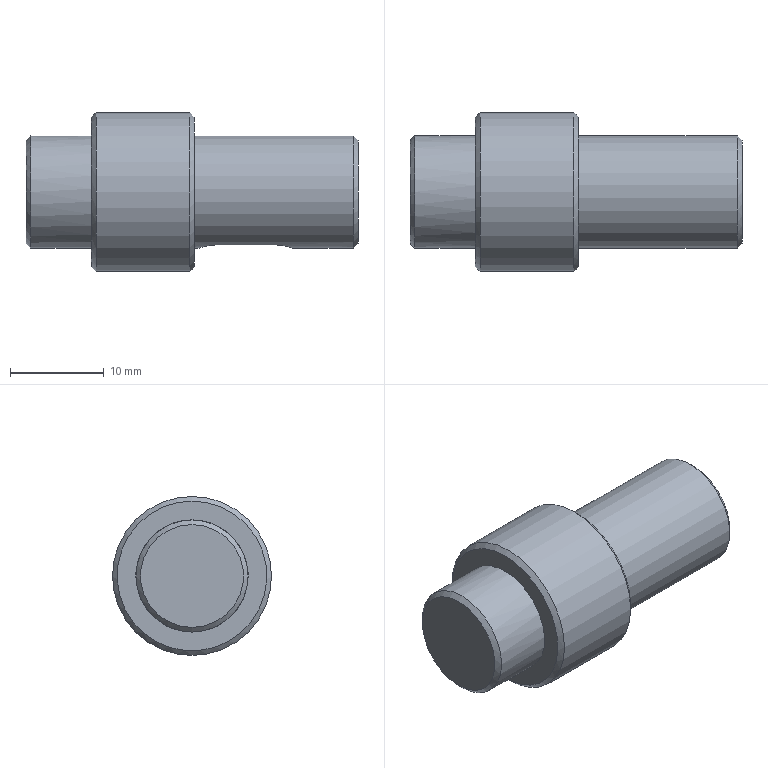Part | NX | features BREP 1 | 1 solid | 16 faces | box 35.5 x 17 x 17 mm | volume 5158 mm3 | plane 7 | cylinder 5 | cone 4 | commonest cylinder face diameters 4 x2 12 x2 17 x1
STEP:
#1=CARTESIAN_POINT('',(35.,0.,-6.));
#2=VERTEX_POINT('',#1);
#3=CARTESIAN_POINT('',(35.,0.,0.));
#4=DIRECTION('',(-1.,0.,0.));
#5=DIRECTION('',(0.,0.,-1.));
#6=AXIS2_PLACEMENT_3D('',#3,#4,#5);
#7=CIRCLE('',#6,6.);
#8=EDGE_CURVE('',#2,#2,#7,.T.);
#9=ORIENTED_EDGE('',*,*,#8,.F.);
#10=EDGE_LOOP('',(#9));
#11=FACE_BOUND('',#10,.T.);
#12=CARTESIAN_POINT('',(35.5,0.,-5.5));
#13=VERTEX_POINT('',#12);
#14=CARTESIAN_POINT('',(35.5,0.,0.));
#15=DIRECTION('',(1.,0.,0.));
#16=DIRECTION('',(0.,0.,-1.));
#17=AXIS2_PLACEMENT_3D('',#14,#15,#16);
#18=CIRCLE('',#17,5.5);
#19=EDGE_CURVE('',#13,#13,#18,.T.);
#20=ORIENTED_EDGE('',*,*,#19,.F.);
#21=EDGE_LOOP('',(#20));
#22=FACE_BOUND('',#21,.T.);
#23=CARTESIAN_POINT('',(35.5,0.,0.));
#24=DIRECTION('',(-1.,0.,0.));
#25=DIRECTION('',(0.,0.,1.));
#26=AXIS2_PLACEMENT_3D('',#23,#24,#25);
#27=CONICAL_SURFACE('',#26,5.5,0.7854);
#28=ADVANCED_FACE('',(#11,#22),#27,.T.);
#29=CARTESIAN_POINT('',(17.5,0.,-8.5));
#30=VERTEX_POINT('',#29);
#31=CARTESIAN_POINT('',(17.5,0.,0.));
#32=DIRECTION('',(-1.,0.,0.));
#33=DIRECTION('',(0.,0.,-1.));
#34=AXIS2_PLACEMENT_3D('',#31,#32,#33);
#35=CIRCLE('',#34,8.5);
#36=EDGE_CURVE('',#30,#30,#35,.T.);
#37=ORIENTED_EDGE('',*,*,#36,.F.);
#38=EDGE_LOOP('',(#37));
#39=FACE_BOUND('',#38,.T.);
#40=CARTESIAN_POINT('',(18.,0.,-8.));
#41=VERTEX_POINT('',#40);
#42=CARTESIAN_POINT('',(18.,0.,0.));
#43=DIRECTION('',(1.,0.,0.));
#44=DIRECTION('',(0.,0.,-1.));
#45=AXIS2_PLACEMENT_3D('',#42,#43,#44);
#46=CIRCLE('',#45,8.);
#47=EDGE_CURVE('',#41,#41,#46,.T.);
#48=ORIENTED_EDGE('',*,*,#47,.F.);
#49=EDGE_LOOP('',(#48));
#50=FACE_BOUND('',#49,.T.);
#51=CARTESIAN_POINT('',(18.,0.,0.));
#52=DIRECTION('',(-1.,0.,0.));
#53=DIRECTION('',(0.,0.,1.));
#54=AXIS2_PLACEMENT_3D('',#51,#52,#53);
#55=CONICAL_SURFACE('',#54,8.,0.7854);
#56=ADVANCED_FACE('',(#39,#50),#55,.T.);
#57=CARTESIAN_POINT('',(7.5,0.,8.5));
#58=VERTEX_POINT('',#57);
#59=CARTESIAN_POINT('',(7.5,0.,0.));
#60=DIRECTION('',(1.,0.,0.));
#61=DIRECTION('',(0.,0.,1.));
#62=AXIS2_PLACEMENT_3D('',#59,#60,#61);
#63=CIRCLE('',#62,8.5);
#64=EDGE_CURVE('',#58,#58,#63,.T.);
#65=ORIENTED_EDGE('',*,*,#64,.F.);
#66=EDGE_LOOP('',(#65));
#67=FACE_BOUND('',#66,.T.);
#68=CARTESIAN_POINT('',(7.,0.,8.));
#69=VERTEX_POINT('',#68);
#70=CARTESIAN_POINT('',(7.,0.,0.));
#71=DIRECTION('',(-1.,0.,0.));
#72=DIRECTION('',(0.,0.,1.));
#73=AXIS2_PLACEMENT_3D('',#70,#71,#72);
#74=CIRCLE('',#73,8.);
#75=EDGE_CURVE('',#69,#69,#74,.T.);
#76=ORIENTED_EDGE('',*,*,#75,.F.);
#77=EDGE_LOOP('',(#76));
#78=FACE_BOUND('',#77,.T.);
#79=CARTESIAN_POINT('',(7.5,0.,0.));
#80=DIRECTION('',(1.,0.,0.));
#81=DIRECTION('',(0.,0.,-1.));
#82=AXIS2_PLACEMENT_3D('',#79,#80,#81);
#83=CONICAL_SURFACE('',#82,8.5,0.7854);
#84=ADVANCED_FACE('',(#67,#78),#83,.T.);
#85=CARTESIAN_POINT('',(0.5,0.,6.));
#86=VERTEX_POINT('',#85);
#87=CARTESIAN_POINT('',(0.5,0.,0.));
#88=DIRECTION('',(1.,0.,0.));
#89=DIRECTION('',(0.,0.,1.));
#90=AXIS2_PLACEMENT_3D('',#87,#88,#89);
#91=CIRCLE('',#90,6.);
#92=EDGE_CURVE('',#86,#86,#91,.T.);
#93=ORIENTED_EDGE('',*,*,#92,.F.);
#94=EDGE_LOOP('',(#93));
#95=FACE_BOUND('',#94,.T.);
#96=CARTESIAN_POINT('',(0.,0.,5.5));
#97=VERTEX_POINT('',#96);
#98=CARTESIAN_POINT('',(0.,0.,0.));
#99=DIRECTION('',(-1.,0.,0.));
#100=DIRECTION('',(0.,0.,1.));
#101=AXIS2_PLACEMENT_3D('',#98,#99,#100);
#102=CIRCLE('',#101,5.5);
#103=EDGE_CURVE('',#97,#97,#102,.T.);
#104=ORIENTED_EDGE('',*,*,#103,.F.);
#105=EDGE_LOOP('',(#104));
#106=FACE_BOUND('',#105,.T.);
#107=CARTESIAN_POINT('',(0.5,0.,0.));
#108=DIRECTION('',(1.,0.,0.));
#109=DIRECTION('',(0.,0.,-1.));
#110=AXIS2_PLACEMENT_3D('',#107,#108,#109);
#111=CONICAL_SURFACE('',#110,6.,0.7854);
#112=ADVANCED_FACE('',(#95,#106),#111,.T.);
#113=CARTESIAN_POINT('',(20.5,-2.,-3.5));
#114=VERTEX_POINT('',#113);
#115=CARTESIAN_POINT('',(20.5,2.,-3.5));
#116=VERTEX_POINT('',#115);
#117=CARTESIAN_POINT('',(20.5,0.,-3.5));
#118=DIRECTION('',(0.,0.,-1.));
#119=DIRECTION('',(1.,0.,0.));
#120=AXIS2_PLACEMENT_3D('',#117,#118,#119);
#121=CIRCLE('',#120,2.);
#122=EDGE_CURVE('',#114,#116,#121,.T.);
#123=ORIENTED_EDGE('',*,*,#122,.F.);
#124=CARTESIAN_POINT('',(20.5,-2.,-5.657));
#125=VERTEX_POINT('',#124);
#126=CARTESIAN_POINT('',(20.5,-2.,-3.5));
#127=DIRECTION('',(0.,0.,-1.));
#128=VECTOR('',#127,1000.);
#129=LINE('',#126,#128);
#130=EDGE_CURVE('',#114,#125,#129,.T.);
#131=ORIENTED_EDGE('',*,*,#130,.T.);
#132=CARTESIAN_POINT('',(20.5,2.,-5.657));
#133=VERTEX_POINT('',#132);
#134=CARTESIAN_POINT('',(20.5,-2.,-5.657));
#135=CARTESIAN_POINT('',(19.967,-2.,-5.657));
#136=CARTESIAN_POINT('',(18.938,-1.567,-5.833));
#137=CARTESIAN_POINT('',(18.281,-0.003461,-6.083));
#138=CARTESIAN_POINT('',(18.937,1.568,-5.834));
#139=CARTESIAN_POINT('',(19.967,2.,-5.657));
#140=CARTESIAN_POINT('',(20.5,2.,-5.657));
#141=B_SPLINE_CURVE_WITH_KNOTS('',3,(#134,#135,#136,#137,#138,#139,#140),.UNSPECIFIED.,.F.,.F.,(4,1,1,1,4),(0.,0.001574,0.003148,0.004722,0.006296),.UNSPECIFIED.);
#142=EDGE_CURVE('',#125,#133,#141,.T.);
#143=ORIENTED_EDGE('',*,*,#142,.T.);
#144=CARTESIAN_POINT('',(20.5,2.,-3.5));
#145=DIRECTION('',(0.,0.,-1.));
#146=VECTOR('',#145,1000.);
#147=LINE('',#144,#146);
#148=EDGE_CURVE('',#116,#133,#147,.T.);
#149=ORIENTED_EDGE('',*,*,#148,.F.);
#150=EDGE_LOOP('',(#123,#131,#143,#149));
#151=FACE_BOUND('',#150,.T.);
#152=CARTESIAN_POINT('',(20.5,0.,-3.5));
#153=DIRECTION('',(0.,0.,-1.));
#154=DIRECTION('',(-1.,0.,0.));
#155=AXIS2_PLACEMENT_3D('',#152,#153,#154);
#156=CYLINDRICAL_SURFACE('',#155,2.);
#157=ADVANCED_FACE('',(#151),#156,.F.);
#158=ORIENTED_EDGE('',*,*,#8,.T.);
#159=EDGE_LOOP('',(#158));
#160=FACE_BOUND('',#159,.T.);
#161=ORIENTED_EDGE('',*,*,#142,.F.);
#162=CARTESIAN_POINT('',(26.5,-2.,-5.657));
#163=VERTEX_POINT('',#162);
#164=CARTESIAN_POINT('',(35.5,-2.,-5.657));
#165=DIRECTION('',(-1.,0.,0.));
#166=VECTOR('',#165,1000.);
#167=LINE('',#164,#166);
#168=EDGE_CURVE('',#163,#125,#167,.T.);
#169=ORIENTED_EDGE('',*,*,#168,.F.);
#170=CARTESIAN_POINT('',(26.5,2.,-5.657));
#171=VERTEX_POINT('',#170);
#172=CARTESIAN_POINT('',(26.5,2.,-5.657));
#173=CARTESIAN_POINT('',(27.033,2.,-5.657));
#174=CARTESIAN_POINT('',(28.062,1.567,-5.833));
#175=CARTESIAN_POINT('',(28.719,0.003461,-6.083));
#176=CARTESIAN_POINT('',(28.063,-1.568,-5.834));
#177=CARTESIAN_POINT('',(27.033,-2.,-5.657));
#178=CARTESIAN_POINT('',(26.5,-2.,-5.657));
#179=B_SPLINE_CURVE_WITH_KNOTS('',3,(#172,#173,#174,#175,#176,#177,#178),.UNSPECIFIED.,.F.,.F.,(4,1,1,1,4),(0.,0.001574,0.003148,0.004722,0.006296),.UNSPECIFIED.);
#180=EDGE_CURVE('',#171,#163,#179,.T.);
#181=ORIENTED_EDGE('',*,*,#180,.F.);
#182=CARTESIAN_POINT('',(35.5,2.,-5.657));
#183=DIRECTION('',(1.,0.,0.));
#184=VECTOR('',#183,1000.);
#185=LINE('',#182,#184);
#186=EDGE_CURVE('',#133,#171,#185,.T.);
#187=ORIENTED_EDGE('',*,*,#186,.F.);
#188=EDGE_LOOP('',(#161,#169,#181,#187));
#189=FACE_BOUND('',#188,.T.);
#190=CARTESIAN_POINT('',(18.,0.,-6.));
#191=VERTEX_POINT('',#190);
#192=CARTESIAN_POINT('',(18.,0.,0.));
#193=DIRECTION('',(1.,0.,0.));
#194=DIRECTION('',(0.,0.,-1.));
#195=AXIS2_PLACEMENT_3D('',#192,#193,#194);
#196=CIRCLE('',#195,6.);
#197=EDGE_CURVE('',#191,#191,#196,.T.);
#198=ORIENTED_EDGE('',*,*,#197,.T.);
#199=EDGE_LOOP('',(#198));
#200=FACE_BOUND('',#199,.T.);
#201=CARTESIAN_POINT('',(35.5,0.,0.));
#202=DIRECTION('',(1.,0.,0.));
#203=DIRECTION('',(0.,0.,-1.));
#204=AXIS2_PLACEMENT_3D('',#201,#202,#203);
#205=CYLINDRICAL_SURFACE('',#204,6.);
#206=ADVANCED_FACE('',(#160,#189,#200),#205,.T.);
#207=ORIENTED_EDGE('',*,*,#36,.T.);
#208=EDGE_LOOP('',(#207));
#209=FACE_BOUND('',#208,.T.);
#210=ORIENTED_EDGE('',*,*,#64,.T.);
#211=EDGE_LOOP('',(#210));
#212=FACE_BOUND('',#211,.T.);
#213=CARTESIAN_POINT('',(35.5,0.,0.));
#214=DIRECTION('',(1.,0.,0.));
#215=DIRECTION('',(0.,0.,-1.));
#216=AXIS2_PLACEMENT_3D('',#213,#214,#215);
#217=CYLINDRICAL_SURFACE('',#216,8.5);
#218=ADVANCED_FACE('',(#209,#212),#217,.T.);
#219=CARTESIAN_POINT('',(7.,0.,-6.));
#220=VERTEX_POINT('',#219);
#221=CARTESIAN_POINT('',(7.,0.,0.));
#222=DIRECTION('',(1.,0.,0.));
#223=DIRECTION('',(0.,0.,-1.));
#224=AXIS2_PLACEMENT_3D('',#221,#222,#223);
#225=CIRCLE('',#224,6.);
#226=EDGE_CURVE('',#220,#220,#225,.T.);
#227=ORIENTED_EDGE('',*,*,#226,.F.);
#228=EDGE_LOOP('',(#227));
#229=FACE_BOUND('',#228,.T.);
#230=ORIENTED_EDGE('',*,*,#92,.T.);
#231=EDGE_LOOP('',(#230));
#232=FACE_BOUND('',#231,.T.);
#233=CARTESIAN_POINT('',(35.5,0.,0.));
#234=DIRECTION('',(1.,0.,0.));
#235=DIRECTION('',(0.,0.,-1.));
#236=AXIS2_PLACEMENT_3D('',#233,#234,#235);
#237=CYLINDRICAL_SURFACE('',#236,6.);
#238=ADVANCED_FACE('',(#229,#232),#237,.T.);
#239=ORIENTED_EDGE('',*,*,#103,.T.);
#240=EDGE_LOOP('',(#239));
#241=FACE_BOUND('',#240,.T.);
#242=CARTESIAN_POINT('',(0.,0.,0.));
#243=DIRECTION('',(-1.,0.,0.));
#244=DIRECTION('',(0.,0.,1.));
#245=AXIS2_PLACEMENT_3D('',#242,#243,#244);
#246=PLANE('',#245);
#247=ADVANCED_FACE('',(#241),#246,.T.);
#248=ORIENTED_EDGE('',*,*,#75,.T.);
#249=EDGE_LOOP('',(#248));
#250=FACE_BOUND('',#249,.T.);
#251=ORIENTED_EDGE('',*,*,#226,.T.);
#252=EDGE_LOOP('',(#251));
#253=FACE_BOUND('',#252,.T.);
#254=CARTESIAN_POINT('',(7.,6.,0.));
#255=DIRECTION('',(-1.,0.,0.));
#256=DIRECTION('',(0.,0.,1.));
#257=AXIS2_PLACEMENT_3D('',#254,#255,#256);
#258=PLANE('',#257);
#259=ADVANCED_FACE('',(#250,#253),#258,.T.);
#260=ORIENTED_EDGE('',*,*,#47,.T.);
#261=EDGE_LOOP('',(#260));
#262=FACE_BOUND('',#261,.T.);
#263=ORIENTED_EDGE('',*,*,#197,.F.);
#264=EDGE_LOOP('',(#263));
#265=FACE_BOUND('',#264,.T.);
#266=CARTESIAN_POINT('',(18.,8.5,0.));
#267=DIRECTION('',(1.,0.,0.));
#268=DIRECTION('',(0.,0.,-1.));
#269=AXIS2_PLACEMENT_3D('',#266,#267,#268);
#270=PLANE('',#269);
#271=ADVANCED_FACE('',(#262,#265),#270,.T.);
#272=ORIENTED_EDGE('',*,*,#19,.T.);
#273=EDGE_LOOP('',(#272));
#274=FACE_BOUND('',#273,.T.);
#275=CARTESIAN_POINT('',(35.5,6.,0.));
#276=DIRECTION('',(1.,0.,0.));
#277=DIRECTION('',(0.,0.,-1.));
#278=AXIS2_PLACEMENT_3D('',#275,#276,#277);
#279=PLANE('',#278);
#280=ADVANCED_FACE('',(#274),#279,.T.);
#281=CARTESIAN_POINT('',(26.5,2.,-3.5));
#282=VERTEX_POINT('',#281);
#283=CARTESIAN_POINT('',(26.5,2.,-3.5));
#284=DIRECTION('',(0.,0.,-1.));
#285=VECTOR('',#284,1000.);
#286=LINE('',#283,#285);
#287=EDGE_CURVE('',#282,#171,#286,.T.);
#288=ORIENTED_EDGE('',*,*,#287,.T.);
#289=ORIENTED_EDGE('',*,*,#180,.T.);
#290=CARTESIAN_POINT('',(26.5,-2.,-3.5));
#291=VERTEX_POINT('',#290);
#292=CARTESIAN_POINT('',(26.5,-2.,-3.5));
#293=DIRECTION('',(0.,0.,-1.));
#294=VECTOR('',#293,1000.);
#295=LINE('',#292,#294);
#296=EDGE_CURVE('',#291,#163,#295,.T.);
#297=ORIENTED_EDGE('',*,*,#296,.F.);
#298=CARTESIAN_POINT('',(26.5,0.,-3.5));
#299=DIRECTION('',(0.,0.,-1.));
#300=DIRECTION('',(-1.,0.,0.));
#301=AXIS2_PLACEMENT_3D('',#298,#299,#300);
#302=CIRCLE('',#301,2.);
#303=EDGE_CURVE('',#282,#291,#302,.T.);
#304=ORIENTED_EDGE('',*,*,#303,.F.);
#305=EDGE_LOOP('',(#288,#289,#297,#304));
#306=FACE_BOUND('',#305,.T.);
#307=CARTESIAN_POINT('',(26.5,0.,-3.5));
#308=DIRECTION('',(0.,0.,-1.));
#309=DIRECTION('',(-1.,0.,0.));
#310=AXIS2_PLACEMENT_3D('',#307,#308,#309);
#311=CYLINDRICAL_SURFACE('',#310,2.);
#312=ADVANCED_FACE('',(#306),#311,.F.);
#313=ORIENTED_EDGE('',*,*,#186,.T.);
#314=ORIENTED_EDGE('',*,*,#287,.F.);
#315=CARTESIAN_POINT('',(26.5,2.,-3.5));
#316=DIRECTION('',(1.,0.,0.));
#317=VECTOR('',#316,1000.);
#318=LINE('',#315,#317);
#319=EDGE_CURVE('',#116,#282,#318,.T.);
#320=ORIENTED_EDGE('',*,*,#319,.F.);
#321=ORIENTED_EDGE('',*,*,#148,.T.);
#322=EDGE_LOOP('',(#313,#314,#320,#321));
#323=FACE_BOUND('',#322,.T.);
#324=CARTESIAN_POINT('',(26.5,2.,-3.5));
#325=DIRECTION('',(0.,1.,0.));
#326=DIRECTION('',(0.,0.,1.));
#327=AXIS2_PLACEMENT_3D('',#324,#325,#326);
#328=PLANE('',#327);
#329=ADVANCED_FACE('',(#323),#328,.F.);
#330=ORIENTED_EDGE('',*,*,#168,.T.);
#331=ORIENTED_EDGE('',*,*,#130,.F.);
#332=CARTESIAN_POINT('',(26.5,-2.,-3.5));
#333=DIRECTION('',(-1.,0.,0.));
#334=VECTOR('',#333,1000.);
#335=LINE('',#332,#334);
#336=EDGE_CURVE('',#291,#114,#335,.T.);
#337=ORIENTED_EDGE('',*,*,#336,.F.);
#338=ORIENTED_EDGE('',*,*,#296,.T.);
#339=EDGE_LOOP('',(#330,#331,#337,#338));
#340=FACE_BOUND('',#339,.T.);
#341=CARTESIAN_POINT('',(26.5,-2.,-3.5));
#342=DIRECTION('',(0.,-1.,0.));
#343=DIRECTION('',(0.,0.,-1.));
#344=AXIS2_PLACEMENT_3D('',#341,#342,#343);
#345=PLANE('',#344);
#346=ADVANCED_FACE('',(#340),#345,.F.);
#347=ORIENTED_EDGE('',*,*,#303,.T.);
#348=ORIENTED_EDGE('',*,*,#336,.T.);
#349=ORIENTED_EDGE('',*,*,#122,.T.);
#350=ORIENTED_EDGE('',*,*,#319,.T.);
#351=EDGE_LOOP('',(#347,#348,#349,#350));
#352=FACE_BOUND('',#351,.T.);
#353=CARTESIAN_POINT('',(26.5,0.,-3.5));
#354=DIRECTION('',(0.,0.,-1.));
#355=DIRECTION('',(-1.,0.,0.));
#356=AXIS2_PLACEMENT_3D('',#353,#354,#355);
#357=PLANE('',#356);
#358=ADVANCED_FACE('',(#352),#357,.T.);
#359=CLOSED_SHELL('',(#28,#56,#84,#112,#157,#206,#218,#238,#247,#259,#271,#280,#312,#329,#346,#358));
#360=MANIFOLD_SOLID_BREP('',#359);
#361=(LENGTH_UNIT()NAMED_UNIT(*)SI_UNIT(.MILLI.,.METRE.));
#362=UNCERTAINTY_MEASURE_WITH_UNIT(LENGTH_MEASURE(0.0508),#361,'','');
#363=(NAMED_UNIT(*)PLANE_ANGLE_UNIT()SI_UNIT($,.RADIAN.));
#364=(NAMED_UNIT(*)SI_UNIT($,.STERADIAN.)SOLID_ANGLE_UNIT());
#365=(GEOMETRIC_REPRESENTATION_CONTEXT(3)GLOBAL_UNCERTAINTY_ASSIGNED_CONTEXT((#362))GLOBAL_UNIT_ASSIGNED_CONTEXT((#361,#363,#364))REPRESENTATION_CONTEXT('',''));
#366=ADVANCED_BREP_SHAPE_REPRESENTATION('',(#360),#365);